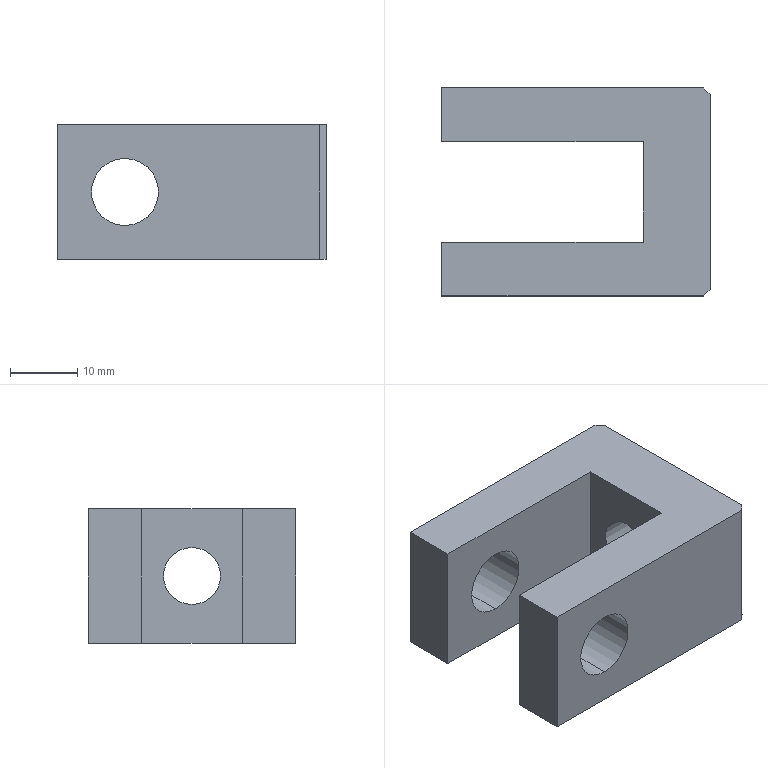Part | SolidWorks | features HoleWzd 3, Chamfer 1, Extrusion 1, ICE 1 | 1 solid | 18 faces | box 40 x 31 x 20 mm | volume 13956 mm3 | plane 12 | cylinder 6 | commonest cylinder face diameters 10 x4 8.5 x2
STEP:
#1=CARTESIAN_POINT('',(-6.962,15.5,5.));
#2=VERTEX_POINT('',#1);
#3=CARTESIAN_POINT('',(-6.962,15.5,-5.));
#4=VERTEX_POINT('',#3);
#5=CARTESIAN_POINT('',(-6.962,15.5,0.));
#6=DIRECTION('',(0.,-1.,0.));
#7=DIRECTION('',(0.,0.,-1.));
#8=AXIS2_PLACEMENT_3D('',#5,#6,#7);
#9=CIRCLE('',#8,5.);
#10=EDGE_CURVE('',#2,#4,#9,.T.);
#11=ORIENTED_EDGE('',*,*,#10,.F.);
#12=CARTESIAN_POINT('',(-6.962,7.5,5.));
#13=VERTEX_POINT('',#12);
#14=CARTESIAN_POINT('',(-6.962,7.5,5.));
#15=DIRECTION('',(0.,-1.,0.));
#16=VECTOR('',#15,1000.);
#17=LINE('',#14,#16);
#18=EDGE_CURVE('',#2,#13,#17,.T.);
#19=ORIENTED_EDGE('',*,*,#18,.T.);
#20=CARTESIAN_POINT('',(-6.962,7.5,-5.));
#21=VERTEX_POINT('',#20);
#22=CARTESIAN_POINT('',(-6.962,7.5,0.));
#23=DIRECTION('',(0.,-1.,0.));
#24=DIRECTION('',(0.,0.,-1.));
#25=AXIS2_PLACEMENT_3D('',#22,#23,#24);
#26=CIRCLE('',#25,5.);
#27=EDGE_CURVE('',#13,#21,#26,.T.);
#28=ORIENTED_EDGE('',*,*,#27,.T.);
#29=CARTESIAN_POINT('',(-6.962,7.5,-5.));
#30=DIRECTION('',(0.,-1.,0.));
#31=VECTOR('',#30,1000.);
#32=LINE('',#29,#31);
#33=EDGE_CURVE('',#4,#21,#32,.T.);
#34=ORIENTED_EDGE('',*,*,#33,.F.);
#35=EDGE_LOOP('',(#11,#19,#28,#34));
#36=FACE_OUTER_BOUND('',#35,.T.);
#37=CARTESIAN_POINT('',(-6.962,7.5,0.));
#38=DIRECTION('',(0.,-1.,0.));
#39=DIRECTION('',(0.,0.,-1.));
#40=AXIS2_PLACEMENT_3D('',#37,#38,#39);
#41=CYLINDRICAL_SURFACE('',#40,5.);
#42=ADVANCED_FACE('',(#36),#41,.F.);
#43=CARTESIAN_POINT('',(13.038,0.,4.25));
#44=VERTEX_POINT('',#43);
#45=CARTESIAN_POINT('',(13.038,0.,-4.25));
#46=VERTEX_POINT('',#45);
#47=CARTESIAN_POINT('',(13.038,0.,0.));
#48=DIRECTION('',(1.,0.,0.));
#49=DIRECTION('',(0.,0.,-1.));
#50=AXIS2_PLACEMENT_3D('',#47,#48,#49);
#51=CIRCLE('',#50,4.25);
#52=EDGE_CURVE('',#44,#46,#51,.T.);
#53=ORIENTED_EDGE('',*,*,#52,.F.);
#54=CARTESIAN_POINT('',(23.038,0.,4.25));
#55=VERTEX_POINT('',#54);
#56=CARTESIAN_POINT('',(23.038,0.,4.25));
#57=DIRECTION('',(1.,0.,0.));
#58=VECTOR('',#57,1000.);
#59=LINE('',#56,#58);
#60=EDGE_CURVE('',#44,#55,#59,.T.);
#61=ORIENTED_EDGE('',*,*,#60,.T.);
#62=CARTESIAN_POINT('',(23.038,0.,-4.25));
#63=VERTEX_POINT('',#62);
#64=CARTESIAN_POINT('',(23.038,0.,0.));
#65=DIRECTION('',(1.,0.,0.));
#66=DIRECTION('',(0.,0.,-1.));
#67=AXIS2_PLACEMENT_3D('',#64,#65,#66);
#68=CIRCLE('',#67,4.25);
#69=EDGE_CURVE('',#55,#63,#68,.T.);
#70=ORIENTED_EDGE('',*,*,#69,.T.);
#71=CARTESIAN_POINT('',(23.038,0.,-4.25));
#72=DIRECTION('',(1.,0.,0.));
#73=VECTOR('',#72,1000.);
#74=LINE('',#71,#73);
#75=EDGE_CURVE('',#46,#63,#74,.T.);
#76=ORIENTED_EDGE('',*,*,#75,.F.);
#77=EDGE_LOOP('',(#53,#61,#70,#76));
#78=FACE_OUTER_BOUND('',#77,.T.);
#79=CARTESIAN_POINT('',(23.038,0.,0.));
#80=DIRECTION('',(1.,0.,0.));
#81=DIRECTION('',(0.,0.,-1.));
#82=AXIS2_PLACEMENT_3D('',#79,#80,#81);
#83=CYLINDRICAL_SURFACE('',#82,4.25);
#84=ADVANCED_FACE('',(#78),#83,.F.);
#85=CARTESIAN_POINT('',(-6.962,-7.5,5.));
#86=VERTEX_POINT('',#85);
#87=CARTESIAN_POINT('',(-6.962,-7.5,-5.));
#88=VERTEX_POINT('',#87);
#89=CARTESIAN_POINT('',(-6.962,-7.5,0.));
#90=DIRECTION('',(0.,-1.,0.));
#91=DIRECTION('',(0.,0.,-1.));
#92=AXIS2_PLACEMENT_3D('',#89,#90,#91);
#93=CIRCLE('',#92,5.);
#94=EDGE_CURVE('',#86,#88,#93,.T.);
#95=ORIENTED_EDGE('',*,*,#94,.F.);
#96=CARTESIAN_POINT('',(-6.962,-15.5,5.));
#97=VERTEX_POINT('',#96);
#98=CARTESIAN_POINT('',(-6.962,-15.5,5.));
#99=DIRECTION('',(0.,-1.,0.));
#100=VECTOR('',#99,1000.);
#101=LINE('',#98,#100);
#102=EDGE_CURVE('',#86,#97,#101,.T.);
#103=ORIENTED_EDGE('',*,*,#102,.T.);
#104=CARTESIAN_POINT('',(-6.962,-15.5,-5.));
#105=VERTEX_POINT('',#104);
#106=CARTESIAN_POINT('',(-6.962,-15.5,0.));
#107=DIRECTION('',(0.,-1.,0.));
#108=DIRECTION('',(0.,0.,-1.));
#109=AXIS2_PLACEMENT_3D('',#106,#107,#108);
#110=CIRCLE('',#109,5.);
#111=EDGE_CURVE('',#97,#105,#110,.T.);
#112=ORIENTED_EDGE('',*,*,#111,.T.);
#113=CARTESIAN_POINT('',(-6.962,-15.5,-5.));
#114=DIRECTION('',(0.,-1.,0.));
#115=VECTOR('',#114,1000.);
#116=LINE('',#113,#115);
#117=EDGE_CURVE('',#88,#105,#116,.T.);
#118=ORIENTED_EDGE('',*,*,#117,.F.);
#119=EDGE_LOOP('',(#95,#103,#112,#118));
#120=FACE_OUTER_BOUND('',#119,.T.);
#121=CARTESIAN_POINT('',(-6.962,-15.5,0.));
#122=DIRECTION('',(0.,-1.,0.));
#123=DIRECTION('',(0.,0.,-1.));
#124=AXIS2_PLACEMENT_3D('',#121,#122,#123);
#125=CYLINDRICAL_SURFACE('',#124,5.);
#126=ADVANCED_FACE('',(#120),#125,.F.);
#127=CARTESIAN_POINT('',(-16.962,7.5,-10.));
#128=VERTEX_POINT('',#127);
#129=CARTESIAN_POINT('',(-16.962,7.5,10.));
#130=VERTEX_POINT('',#129);
#131=CARTESIAN_POINT('',(-16.962,7.5,-10.));
#132=DIRECTION('',(0.,0.,1.));
#133=VECTOR('',#132,1000.);
#134=LINE('',#131,#133);
#135=EDGE_CURVE('',#128,#130,#134,.T.);
#136=ORIENTED_EDGE('',*,*,#135,.T.);
#137=CARTESIAN_POINT('',(-16.962,15.5,10.));
#138=VERTEX_POINT('',#137);
#139=CARTESIAN_POINT('',(-16.962,-15.5,10.));
#140=DIRECTION('',(0.,1.,0.));
#141=VECTOR('',#140,1000.);
#142=LINE('',#139,#141);
#143=EDGE_CURVE('',#130,#138,#142,.T.);
#144=ORIENTED_EDGE('',*,*,#143,.T.);
#145=CARTESIAN_POINT('',(-16.962,15.5,-10.));
#146=VERTEX_POINT('',#145);
#147=CARTESIAN_POINT('',(-16.962,15.5,10.));
#148=DIRECTION('',(0.,0.,-1.));
#149=VECTOR('',#148,1000.);
#150=LINE('',#147,#149);
#151=EDGE_CURVE('',#138,#146,#150,.T.);
#152=ORIENTED_EDGE('',*,*,#151,.T.);
#153=CARTESIAN_POINT('',(-16.962,-15.5,-10.));
#154=DIRECTION('',(0.,1.,0.));
#155=VECTOR('',#154,1000.);
#156=LINE('',#153,#155);
#157=EDGE_CURVE('',#128,#146,#156,.T.);
#158=ORIENTED_EDGE('',*,*,#157,.F.);
#159=EDGE_LOOP('',(#136,#144,#152,#158));
#160=FACE_OUTER_BOUND('',#159,.T.);
#161=CARTESIAN_POINT('',(-16.962,-15.5,10.));
#162=DIRECTION('',(-1.,0.,0.));
#163=DIRECTION('',(0.,0.,1.));
#164=AXIS2_PLACEMENT_3D('',#161,#162,#163);
#165=PLANE('',#164);
#166=ADVANCED_FACE('',(#160),#165,.T.);
#167=CARTESIAN_POINT('',(-6.962,-15.5,0.));
#168=DIRECTION('',(0.,-1.,0.));
#169=DIRECTION('',(0.,0.,-1.));
#170=AXIS2_PLACEMENT_3D('',#167,#168,#169);
#171=CIRCLE('',#170,5.);
#172=EDGE_CURVE('',#105,#97,#171,.T.);
#173=ORIENTED_EDGE('',*,*,#172,.F.);
#174=ORIENTED_EDGE('',*,*,#111,.F.);
#175=EDGE_LOOP('',(#173,#174));
#176=FACE_BOUND('',#175,.T.);
#177=CARTESIAN_POINT('',(22.038,-15.5,-10.));
#178=VERTEX_POINT('',#177);
#179=CARTESIAN_POINT('',(-16.962,-15.5,-10.));
#180=VERTEX_POINT('',#179);
#181=CARTESIAN_POINT('',(23.038,-15.5,-10.));
#182=DIRECTION('',(-1.,0.,0.));
#183=VECTOR('',#182,1000.);
#184=LINE('',#181,#183);
#185=EDGE_CURVE('',#178,#180,#184,.T.);
#186=ORIENTED_EDGE('',*,*,#185,.F.);
#187=CARTESIAN_POINT('',(22.038,-15.5,10.));
#188=VERTEX_POINT('',#187);
#189=CARTESIAN_POINT('',(22.038,-15.5,10.));
#190=DIRECTION('',(0.,0.,1.));
#191=VECTOR('',#190,1000.);
#192=LINE('',#189,#191);
#193=EDGE_CURVE('',#178,#188,#192,.T.);
#194=ORIENTED_EDGE('',*,*,#193,.T.);
#195=CARTESIAN_POINT('',(-16.962,-15.5,10.));
#196=VERTEX_POINT('',#195);
#197=CARTESIAN_POINT('',(23.038,-15.5,10.));
#198=DIRECTION('',(-1.,0.,0.));
#199=VECTOR('',#198,1000.);
#200=LINE('',#197,#199);
#201=EDGE_CURVE('',#188,#196,#200,.T.);
#202=ORIENTED_EDGE('',*,*,#201,.T.);
#203=CARTESIAN_POINT('',(-16.962,-15.5,10.));
#204=DIRECTION('',(0.,0.,-1.));
#205=VECTOR('',#204,1000.);
#206=LINE('',#203,#205);
#207=EDGE_CURVE('',#196,#180,#206,.T.);
#208=ORIENTED_EDGE('',*,*,#207,.T.);
#209=EDGE_LOOP('',(#186,#194,#202,#208));
#210=FACE_OUTER_BOUND('',#209,.T.);
#211=CARTESIAN_POINT('',(23.038,-15.5,10.));
#212=DIRECTION('',(0.,-1.,0.));
#213=DIRECTION('',(0.,0.,-1.));
#214=AXIS2_PLACEMENT_3D('',#211,#212,#213);
#215=PLANE('',#214);
#216=ADVANCED_FACE('',(#176,#210),#215,.T.);
#217=CARTESIAN_POINT('',(23.038,0.,0.));
#218=DIRECTION('',(1.,0.,0.));
#219=DIRECTION('',(0.,0.,-1.));
#220=AXIS2_PLACEMENT_3D('',#217,#218,#219);
#221=CIRCLE('',#220,4.25);
#222=EDGE_CURVE('',#63,#55,#221,.T.);
#223=ORIENTED_EDGE('',*,*,#222,.F.);
#224=ORIENTED_EDGE('',*,*,#69,.F.);
#225=EDGE_LOOP('',(#223,#224));
#226=FACE_BOUND('',#225,.T.);
#227=CARTESIAN_POINT('',(23.038,14.5,-10.));
#228=VERTEX_POINT('',#227);
#229=CARTESIAN_POINT('',(23.038,-14.5,-10.));
#230=VERTEX_POINT('',#229);
#231=CARTESIAN_POINT('',(23.038,15.5,-10.));
#232=DIRECTION('',(0.,-1.,0.));
#233=VECTOR('',#232,1000.);
#234=LINE('',#231,#233);
#235=EDGE_CURVE('',#228,#230,#234,.T.);
#236=ORIENTED_EDGE('',*,*,#235,.F.);
#237=CARTESIAN_POINT('',(23.038,14.5,10.));
#238=VERTEX_POINT('',#237);
#239=CARTESIAN_POINT('',(23.038,14.5,10.));
#240=DIRECTION('',(0.,0.,1.));
#241=VECTOR('',#240,1000.);
#242=LINE('',#239,#241);
#243=EDGE_CURVE('',#228,#238,#242,.T.);
#244=ORIENTED_EDGE('',*,*,#243,.T.);
#245=CARTESIAN_POINT('',(23.038,-14.5,10.));
#246=VERTEX_POINT('',#245);
#247=CARTESIAN_POINT('',(23.038,15.5,10.));
#248=DIRECTION('',(0.,-1.,0.));
#249=VECTOR('',#248,1000.);
#250=LINE('',#247,#249);
#251=EDGE_CURVE('',#238,#246,#250,.T.);
#252=ORIENTED_EDGE('',*,*,#251,.T.);
#253=CARTESIAN_POINT('',(23.038,-14.5,10.));
#254=DIRECTION('',(0.,0.,-1.));
#255=VECTOR('',#254,1000.);
#256=LINE('',#253,#255);
#257=EDGE_CURVE('',#246,#230,#256,.T.);
#258=ORIENTED_EDGE('',*,*,#257,.T.);
#259=EDGE_LOOP('',(#236,#244,#252,#258));
#260=FACE_OUTER_BOUND('',#259,.T.);
#261=CARTESIAN_POINT('',(23.038,15.5,10.));
#262=DIRECTION('',(1.,0.,0.));
#263=DIRECTION('',(0.,1.,0.));
#264=AXIS2_PLACEMENT_3D('',#261,#262,#263);
#265=PLANE('',#264);
#266=ADVANCED_FACE('',(#226,#260),#265,.T.);
#267=CARTESIAN_POINT('',(-6.962,15.5,0.));
#268=DIRECTION('',(0.,-1.,0.));
#269=DIRECTION('',(0.,0.,-1.));
#270=AXIS2_PLACEMENT_3D('',#267,#268,#269);
#271=CIRCLE('',#270,5.);
#272=EDGE_CURVE('',#4,#2,#271,.T.);
#273=ORIENTED_EDGE('',*,*,#272,.T.);
#274=ORIENTED_EDGE('',*,*,#10,.T.);
#275=EDGE_LOOP('',(#273,#274));
#276=FACE_BOUND('',#275,.T.);
#277=CARTESIAN_POINT('',(22.038,15.5,10.));
#278=VERTEX_POINT('',#277);
#279=CARTESIAN_POINT('',(-16.962,15.5,10.));
#280=DIRECTION('',(1.,0.,0.));
#281=VECTOR('',#280,1000.);
#282=LINE('',#279,#281);
#283=EDGE_CURVE('',#138,#278,#282,.T.);
#284=ORIENTED_EDGE('',*,*,#283,.T.);
#285=CARTESIAN_POINT('',(22.038,15.5,-10.));
#286=VERTEX_POINT('',#285);
#287=CARTESIAN_POINT('',(22.038,15.5,10.));
#288=DIRECTION('',(0.,0.,-1.));
#289=VECTOR('',#288,1000.);
#290=LINE('',#287,#289);
#291=EDGE_CURVE('',#278,#286,#290,.T.);
#292=ORIENTED_EDGE('',*,*,#291,.T.);
#293=CARTESIAN_POINT('',(-16.962,15.5,-10.));
#294=DIRECTION('',(1.,0.,0.));
#295=VECTOR('',#294,1000.);
#296=LINE('',#293,#295);
#297=EDGE_CURVE('',#146,#286,#296,.T.);
#298=ORIENTED_EDGE('',*,*,#297,.F.);
#299=ORIENTED_EDGE('',*,*,#151,.F.);
#300=EDGE_LOOP('',(#284,#292,#298,#299));
#301=FACE_OUTER_BOUND('',#300,.T.);
#302=CARTESIAN_POINT('',(-16.962,15.5,10.));
#303=DIRECTION('',(0.,1.,0.));
#304=DIRECTION('',(0.,0.,1.));
#305=AXIS2_PLACEMENT_3D('',#302,#303,#304);
#306=PLANE('',#305);
#307=ADVANCED_FACE('',(#276,#301),#306,.T.);
#308=CARTESIAN_POINT('',(-16.962,-7.5,-10.));
#309=VERTEX_POINT('',#308);
#310=CARTESIAN_POINT('',(-16.962,-7.5,10.));
#311=VERTEX_POINT('',#310);
#312=CARTESIAN_POINT('',(-16.962,-7.5,-10.));
#313=DIRECTION('',(0.,0.,1.));
#314=VECTOR('',#313,1000.);
#315=LINE('',#312,#314);
#316=EDGE_CURVE('',#309,#311,#315,.T.);
#317=ORIENTED_EDGE('',*,*,#316,.F.);
#318=CARTESIAN_POINT('',(-16.962,-15.5,-10.));
#319=DIRECTION('',(0.,1.,0.));
#320=VECTOR('',#319,1000.);
#321=LINE('',#318,#320);
#322=EDGE_CURVE('',#180,#309,#321,.T.);
#323=ORIENTED_EDGE('',*,*,#322,.F.);
#324=ORIENTED_EDGE('',*,*,#207,.F.);
#325=CARTESIAN_POINT('',(-16.962,-15.5,10.));
#326=DIRECTION('',(0.,1.,0.));
#327=VECTOR('',#326,1000.);
#328=LINE('',#325,#327);
#329=EDGE_CURVE('',#196,#311,#328,.T.);
#330=ORIENTED_EDGE('',*,*,#329,.T.);
#331=EDGE_LOOP('',(#317,#323,#324,#330));
#332=FACE_OUTER_BOUND('',#331,.T.);
#333=CARTESIAN_POINT('',(-16.962,-15.5,10.));
#334=DIRECTION('',(-1.,0.,0.));
#335=DIRECTION('',(0.,0.,1.));
#336=AXIS2_PLACEMENT_3D('',#333,#334,#335);
#337=PLANE('',#336);
#338=ADVANCED_FACE('',(#332),#337,.T.);
#339=ORIENTED_EDGE('',*,*,#251,.F.);
#340=CARTESIAN_POINT('',(22.038,15.5,10.));
#341=DIRECTION('',(-0.7071,0.7071,0.));
#342=VECTOR('',#341,1000.);
#343=LINE('',#340,#342);
#344=EDGE_CURVE('',#238,#278,#343,.T.);
#345=ORIENTED_EDGE('',*,*,#344,.T.);
#346=ORIENTED_EDGE('',*,*,#283,.F.);
#347=ORIENTED_EDGE('',*,*,#143,.F.);
#348=CARTESIAN_POINT('',(13.038,7.5,10.));
#349=VERTEX_POINT('',#348);
#350=CARTESIAN_POINT('',(13.038,7.5,10.));
#351=DIRECTION('',(-1.,0.,0.));
#352=VECTOR('',#351,1000.);
#353=LINE('',#350,#352);
#354=EDGE_CURVE('',#349,#130,#353,.T.);
#355=ORIENTED_EDGE('',*,*,#354,.F.);
#356=CARTESIAN_POINT('',(13.038,-7.5,10.));
#357=VERTEX_POINT('',#356);
#358=CARTESIAN_POINT('',(13.038,-7.5,10.));
#359=DIRECTION('',(0.,1.,0.));
#360=VECTOR('',#359,1000.);
#361=LINE('',#358,#360);
#362=EDGE_CURVE('',#357,#349,#361,.T.);
#363=ORIENTED_EDGE('',*,*,#362,.F.);
#364=CARTESIAN_POINT('',(-16.962,-7.5,10.));
#365=DIRECTION('',(1.,0.,0.));
#366=VECTOR('',#365,1000.);
#367=LINE('',#364,#366);
#368=EDGE_CURVE('',#311,#357,#367,.T.);
#369=ORIENTED_EDGE('',*,*,#368,.F.);
#370=ORIENTED_EDGE('',*,*,#329,.F.);
#371=ORIENTED_EDGE('',*,*,#201,.F.);
#372=CARTESIAN_POINT('',(23.038,-14.5,10.));
#373=DIRECTION('',(0.7071,0.7071,0.));
#374=VECTOR('',#373,1000.);
#375=LINE('',#372,#374);
#376=EDGE_CURVE('',#188,#246,#375,.T.);
#377=ORIENTED_EDGE('',*,*,#376,.T.);
#378=EDGE_LOOP('',(#339,#345,#346,#347,#355,#363,#369,#370,#371,#377));
#379=FACE_OUTER_BOUND('',#378,.T.);
#380=CARTESIAN_POINT('',(0.,0.,10.));
#381=DIRECTION('',(0.,0.,-1.));
#382=DIRECTION('',(-1.,0.,0.));
#383=AXIS2_PLACEMENT_3D('',#380,#381,#382);
#384=PLANE('',#383);
#385=ADVANCED_FACE('',(#379),#384,.F.);
#386=ORIENTED_EDGE('',*,*,#297,.T.);
#387=CARTESIAN_POINT('',(18.769,18.769,-10.));
#388=DIRECTION('',(0.7071,-0.7071,0.));
#389=VECTOR('',#388,1000.);
#390=LINE('',#387,#389);
#391=EDGE_CURVE('',#286,#228,#390,.T.);
#392=ORIENTED_EDGE('',*,*,#391,.T.);
#393=ORIENTED_EDGE('',*,*,#235,.T.);
#394=CARTESIAN_POINT('',(18.769,-18.769,-10.));
#395=DIRECTION('',(-0.7071,-0.7071,0.));
#396=VECTOR('',#395,1000.);
#397=LINE('',#394,#396);
#398=EDGE_CURVE('',#230,#178,#397,.T.);
#399=ORIENTED_EDGE('',*,*,#398,.T.);
#400=ORIENTED_EDGE('',*,*,#185,.T.);
#401=ORIENTED_EDGE('',*,*,#322,.T.);
#402=CARTESIAN_POINT('',(13.038,-7.5,-10.));
#403=VERTEX_POINT('',#402);
#404=CARTESIAN_POINT('',(-16.962,-7.5,-10.));
#405=DIRECTION('',(1.,0.,0.));
#406=VECTOR('',#405,1000.);
#407=LINE('',#404,#406);
#408=EDGE_CURVE('',#309,#403,#407,.T.);
#409=ORIENTED_EDGE('',*,*,#408,.T.);
#410=CARTESIAN_POINT('',(13.038,7.5,-10.));
#411=VERTEX_POINT('',#410);
#412=CARTESIAN_POINT('',(13.038,-7.5,-10.));
#413=DIRECTION('',(0.,1.,0.));
#414=VECTOR('',#413,1000.);
#415=LINE('',#412,#414);
#416=EDGE_CURVE('',#403,#411,#415,.T.);
#417=ORIENTED_EDGE('',*,*,#416,.T.);
#418=CARTESIAN_POINT('',(13.038,7.5,-10.));
#419=DIRECTION('',(-1.,0.,0.));
#420=VECTOR('',#419,1000.);
#421=LINE('',#418,#420);
#422=EDGE_CURVE('',#411,#128,#421,.T.);
#423=ORIENTED_EDGE('',*,*,#422,.T.);
#424=ORIENTED_EDGE('',*,*,#157,.T.);
#425=EDGE_LOOP('',(#386,#392,#393,#399,#400,#401,#409,#417,#423,#424));
#426=FACE_OUTER_BOUND('',#425,.T.);
#427=CARTESIAN_POINT('',(0.,0.,-10.));
#428=DIRECTION('',(0.,0.,-1.));
#429=DIRECTION('',(-1.,0.,0.));
#430=AXIS2_PLACEMENT_3D('',#427,#428,#429);
#431=PLANE('',#430);
#432=ADVANCED_FACE('',(#426),#431,.T.);
#433=CARTESIAN_POINT('',(-6.962,7.5,0.));
#434=DIRECTION('',(0.,-1.,0.));
#435=DIRECTION('',(0.,0.,-1.));
#436=AXIS2_PLACEMENT_3D('',#433,#434,#435);
#437=CIRCLE('',#436,5.);
#438=EDGE_CURVE('',#21,#13,#437,.T.);
#439=ORIENTED_EDGE('',*,*,#438,.F.);
#440=ORIENTED_EDGE('',*,*,#27,.F.);
#441=EDGE_LOOP('',(#439,#440));
#442=FACE_BOUND('',#441,.T.);
#443=ORIENTED_EDGE('',*,*,#354,.T.);
#444=ORIENTED_EDGE('',*,*,#135,.F.);
#445=ORIENTED_EDGE('',*,*,#422,.F.);
#446=CARTESIAN_POINT('',(13.038,7.5,-10.));
#447=DIRECTION('',(0.,0.,1.));
#448=VECTOR('',#447,1000.);
#449=LINE('',#446,#448);
#450=EDGE_CURVE('',#411,#349,#449,.T.);
#451=ORIENTED_EDGE('',*,*,#450,.T.);
#452=EDGE_LOOP('',(#443,#444,#445,#451));
#453=FACE_OUTER_BOUND('',#452,.T.);
#454=CARTESIAN_POINT('',(13.038,7.5,-10.));
#455=DIRECTION('',(0.,1.,0.));
#456=DIRECTION('',(0.,0.,1.));
#457=AXIS2_PLACEMENT_3D('',#454,#455,#456);
#458=PLANE('',#457);
#459=ADVANCED_FACE('',(#442,#453),#458,.F.);
#460=CARTESIAN_POINT('',(13.038,0.,0.));
#461=DIRECTION('',(1.,0.,0.));
#462=DIRECTION('',(0.,0.,-1.));
#463=AXIS2_PLACEMENT_3D('',#460,#461,#462);
#464=CIRCLE('',#463,4.25);
#465=EDGE_CURVE('',#46,#44,#464,.T.);
#466=ORIENTED_EDGE('',*,*,#465,.T.);
#467=ORIENTED_EDGE('',*,*,#52,.T.);
#468=EDGE_LOOP('',(#466,#467));
#469=FACE_BOUND('',#468,.T.);
#470=ORIENTED_EDGE('',*,*,#362,.T.);
#471=ORIENTED_EDGE('',*,*,#450,.F.);
#472=ORIENTED_EDGE('',*,*,#416,.F.);
#473=CARTESIAN_POINT('',(13.038,-7.5,-10.));
#474=DIRECTION('',(0.,0.,1.));
#475=VECTOR('',#474,1000.);
#476=LINE('',#473,#475);
#477=EDGE_CURVE('',#403,#357,#476,.T.);
#478=ORIENTED_EDGE('',*,*,#477,.T.);
#479=EDGE_LOOP('',(#470,#471,#472,#478));
#480=FACE_OUTER_BOUND('',#479,.T.);
#481=CARTESIAN_POINT('',(13.038,-7.5,-10.));
#482=DIRECTION('',(1.,0.,0.));
#483=DIRECTION('',(0.,0.,-1.));
#484=AXIS2_PLACEMENT_3D('',#481,#482,#483);
#485=PLANE('',#484);
#486=ADVANCED_FACE('',(#469,#480),#485,.F.);
#487=CARTESIAN_POINT('',(-6.962,-7.5,0.));
#488=DIRECTION('',(0.,-1.,0.));
#489=DIRECTION('',(0.,0.,-1.));
#490=AXIS2_PLACEMENT_3D('',#487,#488,#489);
#491=CIRCLE('',#490,5.);
#492=EDGE_CURVE('',#88,#86,#491,.T.);
#493=ORIENTED_EDGE('',*,*,#492,.T.);
#494=ORIENTED_EDGE('',*,*,#94,.T.);
#495=EDGE_LOOP('',(#493,#494));
#496=FACE_BOUND('',#495,.T.);
#497=ORIENTED_EDGE('',*,*,#368,.T.);
#498=ORIENTED_EDGE('',*,*,#477,.F.);
#499=ORIENTED_EDGE('',*,*,#408,.F.);
#500=ORIENTED_EDGE('',*,*,#316,.T.);
#501=EDGE_LOOP('',(#497,#498,#499,#500));
#502=FACE_OUTER_BOUND('',#501,.T.);
#503=CARTESIAN_POINT('',(-16.962,-7.5,-10.));
#504=DIRECTION('',(0.,-1.,0.));
#505=DIRECTION('',(0.,0.,-1.));
#506=AXIS2_PLACEMENT_3D('',#503,#504,#505);
#507=PLANE('',#506);
#508=ADVANCED_FACE('',(#496,#502),#507,.F.);
#509=ORIENTED_EDGE('',*,*,#102,.F.);
#510=ORIENTED_EDGE('',*,*,#492,.F.);
#511=ORIENTED_EDGE('',*,*,#117,.T.);
#512=ORIENTED_EDGE('',*,*,#172,.T.);
#513=EDGE_LOOP('',(#509,#510,#511,#512));
#514=FACE_OUTER_BOUND('',#513,.T.);
#515=CARTESIAN_POINT('',(-6.962,-15.5,0.));
#516=DIRECTION('',(0.,-1.,0.));
#517=DIRECTION('',(0.,0.,-1.));
#518=AXIS2_PLACEMENT_3D('',#515,#516,#517);
#519=CYLINDRICAL_SURFACE('',#518,5.);
#520=ADVANCED_FACE('',(#514),#519,.F.);
#521=ORIENTED_EDGE('',*,*,#60,.F.);
#522=ORIENTED_EDGE('',*,*,#465,.F.);
#523=ORIENTED_EDGE('',*,*,#75,.T.);
#524=ORIENTED_EDGE('',*,*,#222,.T.);
#525=EDGE_LOOP('',(#521,#522,#523,#524));
#526=FACE_OUTER_BOUND('',#525,.T.);
#527=CARTESIAN_POINT('',(23.038,0.,0.));
#528=DIRECTION('',(1.,0.,0.));
#529=DIRECTION('',(0.,0.,-1.));
#530=AXIS2_PLACEMENT_3D('',#527,#528,#529);
#531=CYLINDRICAL_SURFACE('',#530,4.25);
#532=ADVANCED_FACE('',(#526),#531,.F.);
#533=ORIENTED_EDGE('',*,*,#18,.F.);
#534=ORIENTED_EDGE('',*,*,#272,.F.);
#535=ORIENTED_EDGE('',*,*,#33,.T.);
#536=ORIENTED_EDGE('',*,*,#438,.T.);
#537=EDGE_LOOP('',(#533,#534,#535,#536));
#538=FACE_OUTER_BOUND('',#537,.T.);
#539=CARTESIAN_POINT('',(-6.962,7.5,0.));
#540=DIRECTION('',(0.,-1.,0.));
#541=DIRECTION('',(0.,0.,-1.));
#542=AXIS2_PLACEMENT_3D('',#539,#540,#541);
#543=CYLINDRICAL_SURFACE('',#542,5.);
#544=ADVANCED_FACE('',(#538),#543,.F.);
#545=ORIENTED_EDGE('',*,*,#344,.F.);
#546=ORIENTED_EDGE('',*,*,#243,.F.);
#547=ORIENTED_EDGE('',*,*,#391,.F.);
#548=ORIENTED_EDGE('',*,*,#291,.F.);
#549=EDGE_LOOP('',(#545,#546,#547,#548));
#550=FACE_OUTER_BOUND('',#549,.T.);
#551=CARTESIAN_POINT('',(22.038,15.5,10.));
#552=DIRECTION('',(-0.7071,-0.7071,0.));
#553=DIRECTION('',(0.,0.,-1.));
#554=AXIS2_PLACEMENT_3D('',#551,#552,#553);
#555=PLANE('',#554);
#556=ADVANCED_FACE('',(#550),#555,.F.);
#557=ORIENTED_EDGE('',*,*,#376,.F.);
#558=ORIENTED_EDGE('',*,*,#193,.F.);
#559=ORIENTED_EDGE('',*,*,#398,.F.);
#560=ORIENTED_EDGE('',*,*,#257,.F.);
#561=EDGE_LOOP('',(#557,#558,#559,#560));
#562=FACE_OUTER_BOUND('',#561,.T.);
#563=CARTESIAN_POINT('',(23.038,-14.5,10.));
#564=DIRECTION('',(-0.7071,0.7071,0.));
#565=DIRECTION('',(0.,0.,-1.));
#566=AXIS2_PLACEMENT_3D('',#563,#564,#565);
#567=PLANE('',#566);
#568=ADVANCED_FACE('',(#562),#567,.F.);
#569=CLOSED_SHELL('',(#42,#84,#126,#166,#216,#266,#307,#338,#385,#432,#459,#486,#508,#520,#532,#544,#556,#568));
#570=MANIFOLD_SOLID_BREP('',#569);
#571=CARTESIAN_POINT('',(0.,0.,0.));
#572=DIRECTION('',(0.,0.,1.));
#573=DIRECTION('',(1.,0.,0.));
#574=AXIS2_PLACEMENT_3D('',#571,#572,#573);
#575=(LENGTH_UNIT()NAMED_UNIT(*)SI_UNIT(.MILLI.,.METRE.));
#576=UNCERTAINTY_MEASURE_WITH_UNIT(LENGTH_MEASURE(0.00001),#575,'','');
#577=(NAMED_UNIT(*)PLANE_ANGLE_UNIT()SI_UNIT($,.RADIAN.));
#578=(NAMED_UNIT(*)SI_UNIT($,.STERADIAN.)SOLID_ANGLE_UNIT());
#579=(GEOMETRIC_REPRESENTATION_CONTEXT(3)GLOBAL_UNCERTAINTY_ASSIGNED_CONTEXT((#576))GLOBAL_UNIT_ASSIGNED_CONTEXT((#575,#577,#578))REPRESENTATION_CONTEXT('',''));
#580=ADVANCED_BREP_SHAPE_REPRESENTATION('',(#570,#574),#579);